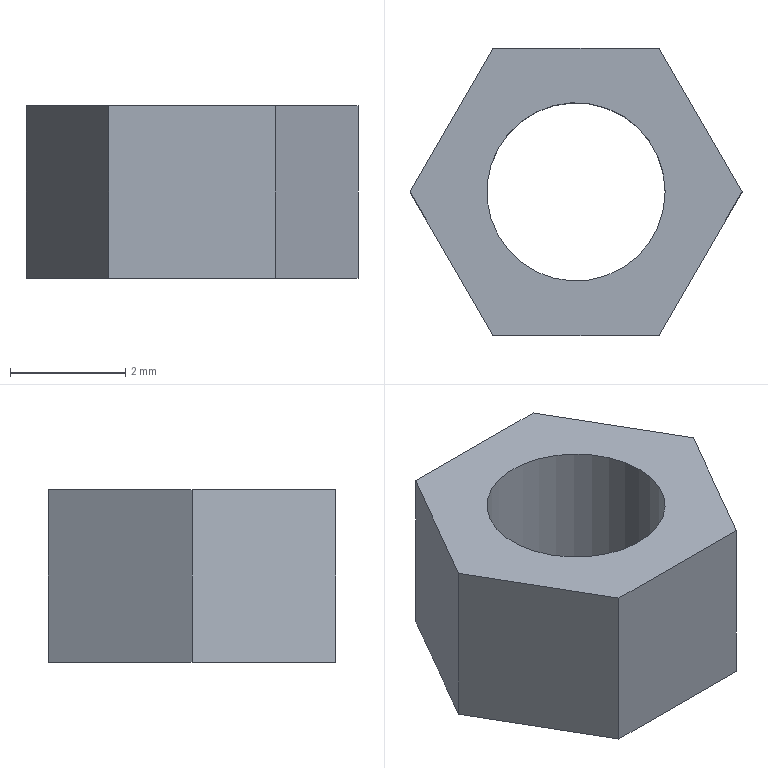Part | NX | features MFD10-WL40_1 2 | 1 solid | 9 faces | box 5.774 x 5 x 3 mm | volume 42.309 mm3 | plane 8 | cylinder 1 | commonest cylinder face diameters 3.1 x1
STEP:
#1=CARTESIAN_POINT('',(241.042,-524.95,94.5));
#2=VERTEX_POINT('',#1);
#3=CARTESIAN_POINT('',(242.485,-522.45,94.5));
#4=VERTEX_POINT('',#3);
#5=CARTESIAN_POINT('',(241.042,-524.95,94.5));
#6=DIRECTION('',(0.5,0.866,0.));
#7=VECTOR('',#6,1000.);
#8=LINE('',#5,#7);
#9=EDGE_CURVE('',#2,#4,#8,.T.);
#10=ORIENTED_EDGE('',*,*,#9,.F.);
#11=CARTESIAN_POINT('',(241.042,-524.95,97.5));
#12=VERTEX_POINT('',#11);
#13=CARTESIAN_POINT('',(241.042,-524.95,97.5));
#14=DIRECTION('',(0.,0.,-1.));
#15=VECTOR('',#14,1000.);
#16=LINE('',#13,#15);
#17=EDGE_CURVE('',#12,#2,#16,.T.);
#18=ORIENTED_EDGE('',*,*,#17,.F.);
#19=CARTESIAN_POINT('',(242.485,-522.45,97.5));
#20=VERTEX_POINT('',#19);
#21=CARTESIAN_POINT('',(241.042,-524.95,97.5));
#22=DIRECTION('',(0.5,0.866,0.));
#23=VECTOR('',#22,1000.);
#24=LINE('',#21,#23);
#25=EDGE_CURVE('',#12,#20,#24,.T.);
#26=ORIENTED_EDGE('',*,*,#25,.T.);
#27=CARTESIAN_POINT('',(242.485,-522.45,97.5));
#28=DIRECTION('',(0.,0.,-1.));
#29=VECTOR('',#28,1000.);
#30=LINE('',#27,#29);
#31=EDGE_CURVE('',#20,#4,#30,.T.);
#32=ORIENTED_EDGE('',*,*,#31,.T.);
#33=EDGE_LOOP('',(#10,#18,#26,#32));
#34=FACE_BOUND('',#33,.T.);
#35=CARTESIAN_POINT('',(241.042,-524.95,97.5));
#36=DIRECTION('',(-0.866,0.5,0.));
#37=DIRECTION('',(-0.5,-0.866,0.));
#38=AXIS2_PLACEMENT_3D('',#35,#36,#37);
#39=PLANE('',#38);
#40=ADVANCED_FACE('',(#34),#39,.T.);
#41=CARTESIAN_POINT('',(245.372,-522.45,94.5));
#42=VERTEX_POINT('',#41);
#43=CARTESIAN_POINT('',(242.485,-522.45,94.5));
#44=DIRECTION('',(1.,0.,0.));
#45=VECTOR('',#44,1000.);
#46=LINE('',#43,#45);
#47=EDGE_CURVE('',#4,#42,#46,.T.);
#48=ORIENTED_EDGE('',*,*,#47,.F.);
#49=ORIENTED_EDGE('',*,*,#31,.F.);
#50=CARTESIAN_POINT('',(245.372,-522.45,97.5));
#51=VERTEX_POINT('',#50);
#52=CARTESIAN_POINT('',(242.485,-522.45,97.5));
#53=DIRECTION('',(1.,0.,0.));
#54=VECTOR('',#53,1000.);
#55=LINE('',#52,#54);
#56=EDGE_CURVE('',#20,#51,#55,.T.);
#57=ORIENTED_EDGE('',*,*,#56,.T.);
#58=CARTESIAN_POINT('',(245.372,-522.45,97.5));
#59=DIRECTION('',(0.,0.,-1.));
#60=VECTOR('',#59,1000.);
#61=LINE('',#58,#60);
#62=EDGE_CURVE('',#51,#42,#61,.T.);
#63=ORIENTED_EDGE('',*,*,#62,.T.);
#64=EDGE_LOOP('',(#48,#49,#57,#63));
#65=FACE_BOUND('',#64,.T.);
#66=CARTESIAN_POINT('',(242.485,-522.45,97.5));
#67=DIRECTION('',(0.,1.,0.));
#68=DIRECTION('',(0.,0.,1.));
#69=AXIS2_PLACEMENT_3D('',#66,#67,#68);
#70=PLANE('',#69);
#71=ADVANCED_FACE('',(#65),#70,.T.);
#72=CARTESIAN_POINT('',(246.815,-524.95,94.5));
#73=VERTEX_POINT('',#72);
#74=CARTESIAN_POINT('',(245.372,-522.45,94.5));
#75=DIRECTION('',(0.5,-0.866,0.));
#76=VECTOR('',#75,1000.);
#77=LINE('',#74,#76);
#78=EDGE_CURVE('',#42,#73,#77,.T.);
#79=ORIENTED_EDGE('',*,*,#78,.F.);
#80=ORIENTED_EDGE('',*,*,#62,.F.);
#81=CARTESIAN_POINT('',(246.815,-524.95,97.5));
#82=VERTEX_POINT('',#81);
#83=CARTESIAN_POINT('',(245.372,-522.45,97.5));
#84=DIRECTION('',(0.5,-0.866,0.));
#85=VECTOR('',#84,1000.);
#86=LINE('',#83,#85);
#87=EDGE_CURVE('',#51,#82,#86,.T.);
#88=ORIENTED_EDGE('',*,*,#87,.T.);
#89=CARTESIAN_POINT('',(246.815,-524.95,97.5));
#90=DIRECTION('',(0.,0.,-1.));
#91=VECTOR('',#90,1000.);
#92=LINE('',#89,#91);
#93=EDGE_CURVE('',#82,#73,#92,.T.);
#94=ORIENTED_EDGE('',*,*,#93,.T.);
#95=EDGE_LOOP('',(#79,#80,#88,#94));
#96=FACE_BOUND('',#95,.T.);
#97=CARTESIAN_POINT('',(245.372,-522.45,97.5));
#98=DIRECTION('',(0.866,0.5,0.));
#99=DIRECTION('',(0.,0.,1.));
#100=AXIS2_PLACEMENT_3D('',#97,#98,#99);
#101=PLANE('',#100);
#102=ADVANCED_FACE('',(#96),#101,.T.);
#103=CARTESIAN_POINT('',(245.372,-527.45,94.5));
#104=VERTEX_POINT('',#103);
#105=CARTESIAN_POINT('',(246.815,-524.95,94.5));
#106=DIRECTION('',(-0.5,-0.866,0.));
#107=VECTOR('',#106,1000.);
#108=LINE('',#105,#107);
#109=EDGE_CURVE('',#73,#104,#108,.T.);
#110=ORIENTED_EDGE('',*,*,#109,.F.);
#111=ORIENTED_EDGE('',*,*,#93,.F.);
#112=CARTESIAN_POINT('',(245.372,-527.45,97.5));
#113=VERTEX_POINT('',#112);
#114=CARTESIAN_POINT('',(246.815,-524.95,97.5));
#115=DIRECTION('',(-0.5,-0.866,0.));
#116=VECTOR('',#115,1000.);
#117=LINE('',#114,#116);
#118=EDGE_CURVE('',#82,#113,#117,.T.);
#119=ORIENTED_EDGE('',*,*,#118,.T.);
#120=CARTESIAN_POINT('',(245.372,-527.45,97.5));
#121=DIRECTION('',(0.,0.,-1.));
#122=VECTOR('',#121,1000.);
#123=LINE('',#120,#122);
#124=EDGE_CURVE('',#113,#104,#123,.T.);
#125=ORIENTED_EDGE('',*,*,#124,.T.);
#126=EDGE_LOOP('',(#110,#111,#119,#125));
#127=FACE_BOUND('',#126,.T.);
#128=CARTESIAN_POINT('',(246.815,-524.95,97.5));
#129=DIRECTION('',(0.866,-0.5,0.));
#130=DIRECTION('',(0.,0.,1.));
#131=AXIS2_PLACEMENT_3D('',#128,#129,#130);
#132=PLANE('',#131);
#133=ADVANCED_FACE('',(#127),#132,.T.);
#134=CARTESIAN_POINT('',(242.485,-527.45,94.5));
#135=VERTEX_POINT('',#134);
#136=CARTESIAN_POINT('',(245.372,-527.45,94.5));
#137=DIRECTION('',(-1.,0.,0.));
#138=VECTOR('',#137,1000.);
#139=LINE('',#136,#138);
#140=EDGE_CURVE('',#104,#135,#139,.T.);
#141=ORIENTED_EDGE('',*,*,#140,.F.);
#142=ORIENTED_EDGE('',*,*,#124,.F.);
#143=CARTESIAN_POINT('',(242.485,-527.45,97.5));
#144=VERTEX_POINT('',#143);
#145=CARTESIAN_POINT('',(245.372,-527.45,97.5));
#146=DIRECTION('',(-1.,0.,0.));
#147=VECTOR('',#146,1000.);
#148=LINE('',#145,#147);
#149=EDGE_CURVE('',#113,#144,#148,.T.);
#150=ORIENTED_EDGE('',*,*,#149,.T.);
#151=CARTESIAN_POINT('',(242.485,-527.45,97.5));
#152=DIRECTION('',(0.,0.,-1.));
#153=VECTOR('',#152,1000.);
#154=LINE('',#151,#153);
#155=EDGE_CURVE('',#144,#135,#154,.T.);
#156=ORIENTED_EDGE('',*,*,#155,.T.);
#157=EDGE_LOOP('',(#141,#142,#150,#156));
#158=FACE_BOUND('',#157,.T.);
#159=CARTESIAN_POINT('',(245.372,-527.45,97.5));
#160=DIRECTION('',(0.,-1.,0.));
#161=DIRECTION('',(1.,0.,0.));
#162=AXIS2_PLACEMENT_3D('',#159,#160,#161);
#163=PLANE('',#162);
#164=ADVANCED_FACE('',(#158),#163,.T.);
#165=CARTESIAN_POINT('',(242.485,-527.45,94.5));
#166=DIRECTION('',(-0.5,0.866,0.));
#167=VECTOR('',#166,1000.);
#168=LINE('',#165,#167);
#169=EDGE_CURVE('',#135,#2,#168,.T.);
#170=ORIENTED_EDGE('',*,*,#169,.F.);
#171=ORIENTED_EDGE('',*,*,#155,.F.);
#172=CARTESIAN_POINT('',(242.485,-527.45,97.5));
#173=DIRECTION('',(-0.5,0.866,0.));
#174=VECTOR('',#173,1000.);
#175=LINE('',#172,#174);
#176=EDGE_CURVE('',#144,#12,#175,.T.);
#177=ORIENTED_EDGE('',*,*,#176,.T.);
#178=ORIENTED_EDGE('',*,*,#17,.T.);
#179=EDGE_LOOP('',(#170,#171,#177,#178));
#180=FACE_BOUND('',#179,.T.);
#181=CARTESIAN_POINT('',(242.485,-527.45,97.5));
#182=DIRECTION('',(-0.866,-0.5,0.));
#183=DIRECTION('',(0.,0.,-1.));
#184=AXIS2_PLACEMENT_3D('',#181,#182,#183);
#185=PLANE('',#184);
#186=ADVANCED_FACE('',(#180),#185,.T.);
#187=ORIENTED_EDGE('',*,*,#25,.F.);
#188=ORIENTED_EDGE('',*,*,#176,.F.);
#189=ORIENTED_EDGE('',*,*,#149,.F.);
#190=ORIENTED_EDGE('',*,*,#118,.F.);
#191=ORIENTED_EDGE('',*,*,#87,.F.);
#192=ORIENTED_EDGE('',*,*,#56,.F.);
#193=EDGE_LOOP('',(#187,#188,#189,#190,#191,#192));
#194=FACE_BOUND('',#193,.T.);
#195=CARTESIAN_POINT('',(245.479,-524.95,97.5));
#196=VERTEX_POINT('',#195);
#197=CARTESIAN_POINT('',(243.929,-524.95,97.5));
#198=DIRECTION('',(0.,0.,-1.));
#199=DIRECTION('',(1.,0.,0.));
#200=AXIS2_PLACEMENT_3D('',#197,#198,#199);
#201=CIRCLE('',#200,1.55);
#202=EDGE_CURVE('',#196,#196,#201,.T.);
#203=ORIENTED_EDGE('',*,*,#202,.T.);
#204=EDGE_LOOP('',(#203));
#205=FACE_BOUND('',#204,.T.);
#206=CARTESIAN_POINT('',(242.485,-522.45,97.5));
#207=DIRECTION('',(0.,0.,-1.));
#208=DIRECTION('',(1.,0.,0.));
#209=AXIS2_PLACEMENT_3D('',#206,#207,#208);
#210=PLANE('',#209);
#211=ADVANCED_FACE('',(#194,#205),#210,.F.);
#212=ORIENTED_EDGE('',*,*,#9,.T.);
#213=ORIENTED_EDGE('',*,*,#47,.T.);
#214=ORIENTED_EDGE('',*,*,#78,.T.);
#215=ORIENTED_EDGE('',*,*,#109,.T.);
#216=ORIENTED_EDGE('',*,*,#140,.T.);
#217=ORIENTED_EDGE('',*,*,#169,.T.);
#218=EDGE_LOOP('',(#212,#213,#214,#215,#216,#217));
#219=FACE_BOUND('',#218,.T.);
#220=CARTESIAN_POINT('',(245.479,-524.95,94.5));
#221=VERTEX_POINT('',#220);
#222=CARTESIAN_POINT('',(243.929,-524.95,94.5));
#223=DIRECTION('',(0.,0.,-1.));
#224=DIRECTION('',(1.,0.,0.));
#225=AXIS2_PLACEMENT_3D('',#222,#223,#224);
#226=CIRCLE('',#225,1.55);
#227=EDGE_CURVE('',#221,#221,#226,.T.);
#228=ORIENTED_EDGE('',*,*,#227,.F.);
#229=EDGE_LOOP('',(#228));
#230=FACE_BOUND('',#229,.T.);
#231=CARTESIAN_POINT('',(242.485,-522.45,94.5));
#232=DIRECTION('',(0.,0.,-1.));
#233=DIRECTION('',(1.,0.,0.));
#234=AXIS2_PLACEMENT_3D('',#231,#232,#233);
#235=PLANE('',#234);
#236=ADVANCED_FACE('',(#219,#230),#235,.T.);
#237=ORIENTED_EDGE('',*,*,#227,.T.);
#238=EDGE_LOOP('',(#237));
#239=FACE_BOUND('',#238,.T.);
#240=ORIENTED_EDGE('',*,*,#202,.F.);
#241=EDGE_LOOP('',(#240));
#242=FACE_BOUND('',#241,.T.);
#243=CARTESIAN_POINT('',(243.929,-524.95,97.5));
#244=DIRECTION('',(0.,0.,1.));
#245=DIRECTION('',(1.,0.,0.));
#246=AXIS2_PLACEMENT_3D('',#243,#244,#245);
#247=CYLINDRICAL_SURFACE('',#246,1.55);
#248=ADVANCED_FACE('',(#239,#242),#247,.F.);
#249=CLOSED_SHELL('',(#40,#71,#102,#133,#164,#186,#211,#236,#248));
#250=MANIFOLD_SOLID_BREP('',#249);
#251=(LENGTH_UNIT()NAMED_UNIT(*)SI_UNIT(.MILLI.,.METRE.));
#252=UNCERTAINTY_MEASURE_WITH_UNIT(LENGTH_MEASURE(0.00001),#251,'','');
#253=(NAMED_UNIT(*)PLANE_ANGLE_UNIT()SI_UNIT($,.RADIAN.));
#254=(NAMED_UNIT(*)SI_UNIT($,.STERADIAN.)SOLID_ANGLE_UNIT());
#255=(GEOMETRIC_REPRESENTATION_CONTEXT(3)GLOBAL_UNCERTAINTY_ASSIGNED_CONTEXT((#252))GLOBAL_UNIT_ASSIGNED_CONTEXT((#251,#253,#254))REPRESENTATION_CONTEXT('',''));
#256=ADVANCED_BREP_SHAPE_REPRESENTATION('',(#250),#255);